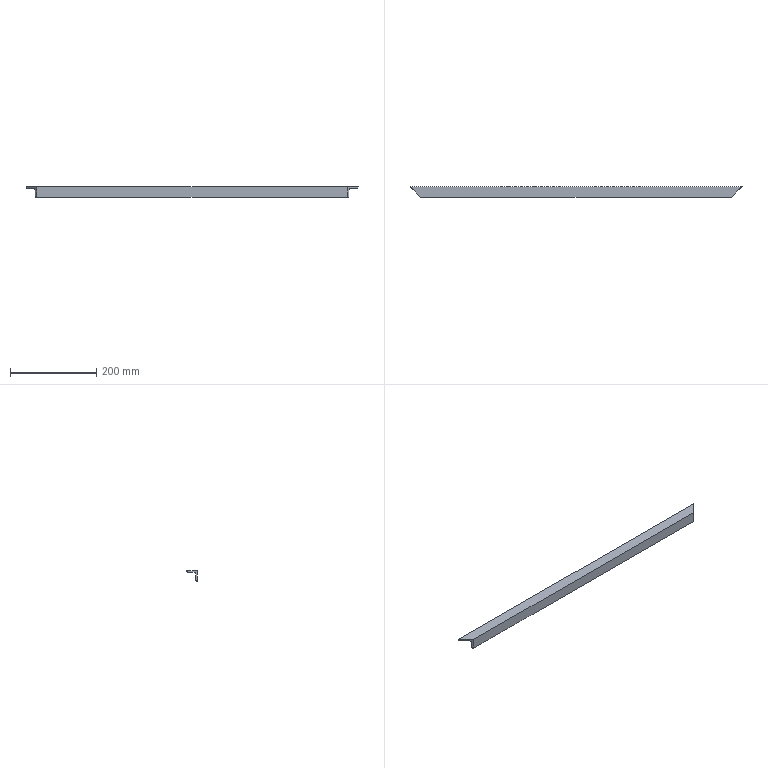Part | STEP file | Guide wheel mechanism revised.sldasm-Part-166 | 1 solid | 9 faces | box 770 x 25 x 25 mm | volume 132103 mm3 | plane 6 | cylinder 3 | commonest cylinder face diameters 8 x2 7 x1
STEP:
#1=CARTESIAN_POINT('',(-360.,1890.,-260.));
#2=VERTEX_POINT('',#1);
#3=CARTESIAN_POINT('',(-385.,1915.,-260.));
#4=VERTEX_POINT('',#3);
#5=CARTESIAN_POINT('',(-372.5,1902.5,-260.));
#6=DIRECTION('',(-0.7071,0.7071,0.));
#7=VECTOR('',#6,1000.);
#8=LINE('',#5,#7);
#9=EDGE_CURVE('',#2,#4,#8,.T.);
#10=ORIENTED_EDGE('',*,*,#9,.F.);
#11=CARTESIAN_POINT('',(360.,1890.,-260.));
#12=VERTEX_POINT('',#11);
#13=CARTESIAN_POINT('',(-360.,1890.,-260.));
#14=DIRECTION('',(1.,0.,0.));
#15=VECTOR('',#14,1000.);
#16=LINE('',#13,#15);
#17=EDGE_CURVE('',#2,#12,#16,.T.);
#18=ORIENTED_EDGE('',*,*,#17,.T.);
#19=CARTESIAN_POINT('',(385.,1915.,-260.));
#20=VERTEX_POINT('',#19);
#21=CARTESIAN_POINT('',(12.5,1542.5,-260.));
#22=DIRECTION('',(-0.7071,-0.7071,0.));
#23=VECTOR('',#22,1000.);
#24=LINE('',#21,#23);
#25=EDGE_CURVE('',#20,#12,#24,.T.);
#26=ORIENTED_EDGE('',*,*,#25,.F.);
#27=CARTESIAN_POINT('',(-360.,1915.,-260.));
#28=DIRECTION('',(1.,0.,0.));
#29=VECTOR('',#28,1000.);
#30=LINE('',#27,#29);
#31=EDGE_CURVE('',#4,#20,#30,.T.);
#32=ORIENTED_EDGE('',*,*,#31,.F.);
#33=EDGE_LOOP('',(#10,#18,#26,#32));
#34=FACE_OUTER_BOUND('',#33,.T.);
#35=CARTESIAN_POINT('',(-360.,1915.,-260.));
#36=DIRECTION('',(0.,0.,-1.));
#37=DIRECTION('',(-1.,0.,0.));
#38=AXIS2_PLACEMENT_3D('',#35,#36,#37);
#39=PLANE('',#38);
#40=ADVANCED_FACE('',(#34),#39,.F.);
#41=CARTESIAN_POINT('',(-381.,1911.,-264.));
#42=VERTEX_POINT('',#41);
#43=CARTESIAN_POINT('',(-385.,1915.,-260.));
#44=CARTESIAN_POINT('',(-385.,1915.,-262.343));
#45=CARTESIAN_POINT('',(-383.343,1913.343,-264.));
#46=CARTESIAN_POINT('',(-381.,1911.,-264.));
#47=(BOUNDED_CURVE()B_SPLINE_CURVE(3,(#43,#44,#45,#46),.UNSPECIFIED.,.F.,.F.)B_SPLINE_CURVE_WITH_KNOTS((4,4),(3.142,4.712),.UNSPECIFIED.)CURVE()GEOMETRIC_REPRESENTATION_ITEM()RATIONAL_B_SPLINE_CURVE((1.,0.8047,0.8047,1.))REPRESENTATION_ITEM(''));
#48=EDGE_CURVE('',#4,#42,#47,.T.);
#49=ORIENTED_EDGE('',*,*,#48,.F.);
#50=ORIENTED_EDGE('',*,*,#31,.T.);
#51=CARTESIAN_POINT('',(381.,1911.,-264.));
#52=VERTEX_POINT('',#51);
#53=CARTESIAN_POINT('',(381.,1911.,-264.));
#54=CARTESIAN_POINT('',(383.343,1913.343,-264.));
#55=CARTESIAN_POINT('',(385.,1915.,-262.343));
#56=CARTESIAN_POINT('',(385.,1915.,-260.));
#57=(BOUNDED_CURVE()B_SPLINE_CURVE(3,(#53,#54,#55,#56),.UNSPECIFIED.,.F.,.F.)B_SPLINE_CURVE_WITH_KNOTS((4,4),(4.712,6.283),.UNSPECIFIED.)CURVE()GEOMETRIC_REPRESENTATION_ITEM()RATIONAL_B_SPLINE_CURVE((1.,0.8047,0.8047,1.))REPRESENTATION_ITEM(''));
#58=EDGE_CURVE('',#52,#20,#57,.T.);
#59=ORIENTED_EDGE('',*,*,#58,.F.);
#60=CARTESIAN_POINT('',(-360.,1911.,-264.));
#61=DIRECTION('',(1.,0.,0.));
#62=VECTOR('',#61,1000.);
#63=LINE('',#60,#62);
#64=EDGE_CURVE('',#42,#52,#63,.T.);
#65=ORIENTED_EDGE('',*,*,#64,.F.);
#66=EDGE_LOOP('',(#49,#50,#59,#65));
#67=FACE_OUTER_BOUND('',#66,.T.);
#68=CARTESIAN_POINT('',(-360.,1911.,-260.));
#69=DIRECTION('',(1.,0.,0.));
#70=DIRECTION('',(0.,0.,-1.));
#71=AXIS2_PLACEMENT_3D('',#68,#69,#70);
#72=CYLINDRICAL_SURFACE('',#71,4.);
#73=ADVANCED_FACE('',(#67),#72,.T.);
#74=CARTESIAN_POINT('',(-367.5,1897.5,-264.));
#75=VERTEX_POINT('',#74);
#76=CARTESIAN_POINT('',(-363.75,1893.75,-264.));
#77=DIRECTION('',(0.7071,-0.7071,0.));
#78=VECTOR('',#77,1000.);
#79=LINE('',#76,#78);
#80=EDGE_CURVE('',#42,#75,#79,.T.);
#81=ORIENTED_EDGE('',*,*,#80,.F.);
#82=ORIENTED_EDGE('',*,*,#64,.T.);
#83=CARTESIAN_POINT('',(367.5,1897.5,-264.));
#84=VERTEX_POINT('',#83);
#85=CARTESIAN_POINT('',(3.75,1533.75,-264.));
#86=DIRECTION('',(0.7071,0.7071,0.));
#87=VECTOR('',#86,1000.);
#88=LINE('',#85,#87);
#89=EDGE_CURVE('',#84,#52,#88,.T.);
#90=ORIENTED_EDGE('',*,*,#89,.F.);
#91=CARTESIAN_POINT('',(-360.,1897.5,-264.));
#92=DIRECTION('',(1.,0.,0.));
#93=VECTOR('',#92,1000.);
#94=LINE('',#91,#93);
#95=EDGE_CURVE('',#75,#84,#94,.T.);
#96=ORIENTED_EDGE('',*,*,#95,.F.);
#97=EDGE_LOOP('',(#81,#82,#90,#96));
#98=FACE_OUTER_BOUND('',#97,.T.);
#99=CARTESIAN_POINT('',(-360.,1897.5,-264.));
#100=DIRECTION('',(0.,0.,1.));
#101=DIRECTION('',(1.,0.,0.));
#102=AXIS2_PLACEMENT_3D('',#99,#100,#101);
#103=PLANE('',#102);
#104=ADVANCED_FACE('',(#98),#103,.F.);
#105=CARTESIAN_POINT('',(-364.,1894.,-267.5));
#106=VERTEX_POINT('',#105);
#107=CARTESIAN_POINT('',(-367.5,1897.5,-264.));
#108=CARTESIAN_POINT('',(-365.45,1895.45,-264.));
#109=CARTESIAN_POINT('',(-364.,1894.,-265.45));
#110=CARTESIAN_POINT('',(-364.,1894.,-267.5));
#111=(BOUNDED_CURVE()B_SPLINE_CURVE(3,(#107,#108,#109,#110),.UNSPECIFIED.,.F.,.F.)B_SPLINE_CURVE_WITH_KNOTS((4,4),(4.712,6.283),.UNSPECIFIED.)CURVE()GEOMETRIC_REPRESENTATION_ITEM()RATIONAL_B_SPLINE_CURVE((1.,0.8047,0.8047,1.))REPRESENTATION_ITEM(''));
#112=EDGE_CURVE('',#75,#106,#111,.T.);
#113=ORIENTED_EDGE('',*,*,#112,.F.);
#114=ORIENTED_EDGE('',*,*,#95,.T.);
#115=CARTESIAN_POINT('',(364.,1894.,-267.5));
#116=VERTEX_POINT('',#115);
#117=CARTESIAN_POINT('',(364.,1894.,-267.5));
#118=CARTESIAN_POINT('',(364.,1894.,-265.45));
#119=CARTESIAN_POINT('',(365.45,1895.45,-264.));
#120=CARTESIAN_POINT('',(367.5,1897.5,-264.));
#121=(BOUNDED_CURVE()B_SPLINE_CURVE(3,(#117,#118,#119,#120),.UNSPECIFIED.,.F.,.F.)B_SPLINE_CURVE_WITH_KNOTS((4,4),(3.142,4.712),.UNSPECIFIED.)CURVE()GEOMETRIC_REPRESENTATION_ITEM()RATIONAL_B_SPLINE_CURVE((1.,0.8047,0.8047,1.))REPRESENTATION_ITEM(''));
#122=EDGE_CURVE('',#116,#84,#121,.T.);
#123=ORIENTED_EDGE('',*,*,#122,.F.);
#124=CARTESIAN_POINT('',(-360.,1894.,-267.5));
#125=DIRECTION('',(1.,0.,0.));
#126=VECTOR('',#125,1000.);
#127=LINE('',#124,#126);
#128=EDGE_CURVE('',#106,#116,#127,.T.);
#129=ORIENTED_EDGE('',*,*,#128,.F.);
#130=EDGE_LOOP('',(#113,#114,#123,#129));
#131=FACE_OUTER_BOUND('',#130,.T.);
#132=CARTESIAN_POINT('',(-360.,1897.5,-267.5));
#133=DIRECTION('',(1.,0.,0.));
#134=DIRECTION('',(0.,0.,-1.));
#135=AXIS2_PLACEMENT_3D('',#132,#133,#134);
#136=CYLINDRICAL_SURFACE('',#135,3.5);
#137=ADVANCED_FACE('',(#131),#136,.F.);
#138=CARTESIAN_POINT('',(-364.,1894.,-281.));
#139=VERTEX_POINT('',#138);
#140=CARTESIAN_POINT('',(-364.,1894.,-281.));
#141=DIRECTION('',(0.,0.,-1.));
#142=VECTOR('',#141,1000.);
#143=LINE('',#140,#142);
#144=EDGE_CURVE('',#106,#139,#143,.T.);
#145=ORIENTED_EDGE('',*,*,#144,.F.);
#146=ORIENTED_EDGE('',*,*,#128,.T.);
#147=CARTESIAN_POINT('',(364.,1894.,-281.));
#148=VERTEX_POINT('',#147);
#149=CARTESIAN_POINT('',(364.,1894.,-281.));
#150=DIRECTION('',(0.,0.,1.));
#151=VECTOR('',#150,1000.);
#152=LINE('',#149,#151);
#153=EDGE_CURVE('',#148,#116,#152,.T.);
#154=ORIENTED_EDGE('',*,*,#153,.F.);
#155=CARTESIAN_POINT('',(-360.,1894.,-281.));
#156=DIRECTION('',(1.,0.,0.));
#157=VECTOR('',#156,1000.);
#158=LINE('',#155,#157);
#159=EDGE_CURVE('',#139,#148,#158,.T.);
#160=ORIENTED_EDGE('',*,*,#159,.F.);
#161=EDGE_LOOP('',(#145,#146,#154,#160));
#162=FACE_OUTER_BOUND('',#161,.T.);
#163=CARTESIAN_POINT('',(-360.,1894.,-281.));
#164=DIRECTION('',(0.,-1.,0.));
#165=DIRECTION('',(0.,0.,-1.));
#166=AXIS2_PLACEMENT_3D('',#163,#164,#165);
#167=PLANE('',#166);
#168=ADVANCED_FACE('',(#162),#167,.F.);
#169=CARTESIAN_POINT('',(-360.,1890.,-285.));
#170=VERTEX_POINT('',#169);
#171=CARTESIAN_POINT('',(-364.,1894.,-281.));
#172=CARTESIAN_POINT('',(-364.,1894.,-283.343));
#173=CARTESIAN_POINT('',(-362.343,1892.343,-285.));
#174=CARTESIAN_POINT('',(-360.,1890.,-285.));
#175=(BOUNDED_CURVE()B_SPLINE_CURVE(3,(#171,#172,#173,#174),.UNSPECIFIED.,.F.,.F.)B_SPLINE_CURVE_WITH_KNOTS((4,4),(3.142,4.712),.UNSPECIFIED.)CURVE()GEOMETRIC_REPRESENTATION_ITEM()RATIONAL_B_SPLINE_CURVE((1.,0.8047,0.8047,1.))REPRESENTATION_ITEM(''));
#176=EDGE_CURVE('',#139,#170,#175,.T.);
#177=ORIENTED_EDGE('',*,*,#176,.F.);
#178=ORIENTED_EDGE('',*,*,#159,.T.);
#179=CARTESIAN_POINT('',(360.,1890.,-285.));
#180=VERTEX_POINT('',#179);
#181=CARTESIAN_POINT('',(360.,1890.,-285.));
#182=CARTESIAN_POINT('',(362.343,1892.343,-285.));
#183=CARTESIAN_POINT('',(364.,1894.,-283.343));
#184=CARTESIAN_POINT('',(364.,1894.,-281.));
#185=(BOUNDED_CURVE()B_SPLINE_CURVE(3,(#181,#182,#183,#184),.UNSPECIFIED.,.F.,.F.)B_SPLINE_CURVE_WITH_KNOTS((4,4),(4.712,6.283),.UNSPECIFIED.)CURVE()GEOMETRIC_REPRESENTATION_ITEM()RATIONAL_B_SPLINE_CURVE((1.,0.8047,0.8047,1.))REPRESENTATION_ITEM(''));
#186=EDGE_CURVE('',#180,#148,#185,.T.);
#187=ORIENTED_EDGE('',*,*,#186,.F.);
#188=CARTESIAN_POINT('',(-360.,1890.,-285.));
#189=DIRECTION('',(1.,0.,0.));
#190=VECTOR('',#189,1000.);
#191=LINE('',#188,#190);
#192=EDGE_CURVE('',#170,#180,#191,.T.);
#193=ORIENTED_EDGE('',*,*,#192,.F.);
#194=EDGE_LOOP('',(#177,#178,#187,#193));
#195=FACE_OUTER_BOUND('',#194,.T.);
#196=CARTESIAN_POINT('',(-360.,1890.,-281.));
#197=DIRECTION('',(1.,0.,0.));
#198=DIRECTION('',(0.,0.,-1.));
#199=AXIS2_PLACEMENT_3D('',#196,#197,#198);
#200=CYLINDRICAL_SURFACE('',#199,4.);
#201=ADVANCED_FACE('',(#195),#200,.T.);
#202=CARTESIAN_POINT('',(-360.,1890.,-260.));
#203=DIRECTION('',(0.,0.,1.));
#204=VECTOR('',#203,1000.);
#205=LINE('',#202,#204);
#206=EDGE_CURVE('',#170,#2,#205,.T.);
#207=ORIENTED_EDGE('',*,*,#206,.F.);
#208=ORIENTED_EDGE('',*,*,#192,.T.);
#209=CARTESIAN_POINT('',(360.,1890.,-260.));
#210=DIRECTION('',(0.,0.,-1.));
#211=VECTOR('',#210,1000.);
#212=LINE('',#209,#211);
#213=EDGE_CURVE('',#12,#180,#212,.T.);
#214=ORIENTED_EDGE('',*,*,#213,.F.);
#215=ORIENTED_EDGE('',*,*,#17,.F.);
#216=EDGE_LOOP('',(#207,#208,#214,#215));
#217=FACE_OUTER_BOUND('',#216,.T.);
#218=CARTESIAN_POINT('',(-360.,1890.,-260.));
#219=DIRECTION('',(0.,1.,0.));
#220=DIRECTION('',(0.,0.,1.));
#221=AXIS2_PLACEMENT_3D('',#218,#219,#220);
#222=PLANE('',#221);
#223=ADVANCED_FACE('',(#217),#222,.F.);
#224=ORIENTED_EDGE('',*,*,#58,.T.);
#225=ORIENTED_EDGE('',*,*,#25,.T.);
#226=ORIENTED_EDGE('',*,*,#213,.T.);
#227=ORIENTED_EDGE('',*,*,#186,.T.);
#228=ORIENTED_EDGE('',*,*,#153,.T.);
#229=ORIENTED_EDGE('',*,*,#122,.T.);
#230=ORIENTED_EDGE('',*,*,#89,.T.);
#231=EDGE_LOOP('',(#224,#225,#226,#227,#228,#229,#230));
#232=FACE_OUTER_BOUND('',#231,.T.);
#233=CARTESIAN_POINT('',(360.,1890.,-260.));
#234=DIRECTION('',(0.7071,-0.7071,0.));
#235=DIRECTION('',(0.7071,0.7071,0.));
#236=AXIS2_PLACEMENT_3D('',#233,#234,#235);
#237=PLANE('',#236);
#238=ADVANCED_FACE('',(#232),#237,.T.);
#239=ORIENTED_EDGE('',*,*,#206,.T.);
#240=ORIENTED_EDGE('',*,*,#9,.T.);
#241=ORIENTED_EDGE('',*,*,#48,.T.);
#242=ORIENTED_EDGE('',*,*,#80,.T.);
#243=ORIENTED_EDGE('',*,*,#112,.T.);
#244=ORIENTED_EDGE('',*,*,#144,.T.);
#245=ORIENTED_EDGE('',*,*,#176,.T.);
#246=EDGE_LOOP('',(#239,#240,#241,#242,#243,#244,#245));
#247=FACE_OUTER_BOUND('',#246,.T.);
#248=CARTESIAN_POINT('',(-360.,1890.,-260.));
#249=DIRECTION('',(-0.7071,-0.7071,0.));
#250=DIRECTION('',(0.7071,-0.7071,0.));
#251=AXIS2_PLACEMENT_3D('',#248,#249,#250);
#252=PLANE('',#251);
#253=ADVANCED_FACE('',(#247),#252,.T.);
#254=CLOSED_SHELL('',(#40,#73,#104,#137,#168,#201,#223,#238,#253));
#255=MANIFOLD_SOLID_BREP('',#254);
#256=CARTESIAN_POINT('',(0.,0.,0.));
#257=DIRECTION('',(0.,0.,1.));
#258=DIRECTION('',(1.,0.,0.));
#259=AXIS2_PLACEMENT_3D('',#256,#257,#258);
#260=(LENGTH_UNIT()NAMED_UNIT(*)SI_UNIT(.MILLI.,.METRE.));
#261=UNCERTAINTY_MEASURE_WITH_UNIT(LENGTH_MEASURE(0.00001),#260,'','');
#262=(NAMED_UNIT(*)PLANE_ANGLE_UNIT()SI_UNIT($,.RADIAN.));
#263=(NAMED_UNIT(*)SI_UNIT($,.STERADIAN.)SOLID_ANGLE_UNIT());
#264=(GEOMETRIC_REPRESENTATION_CONTEXT(3)GLOBAL_UNCERTAINTY_ASSIGNED_CONTEXT((#261))GLOBAL_UNIT_ASSIGNED_CONTEXT((#260,#262,#263))REPRESENTATION_CONTEXT('',''));
#265=ADVANCED_BREP_SHAPE_REPRESENTATION('',(#255,#259),#264);